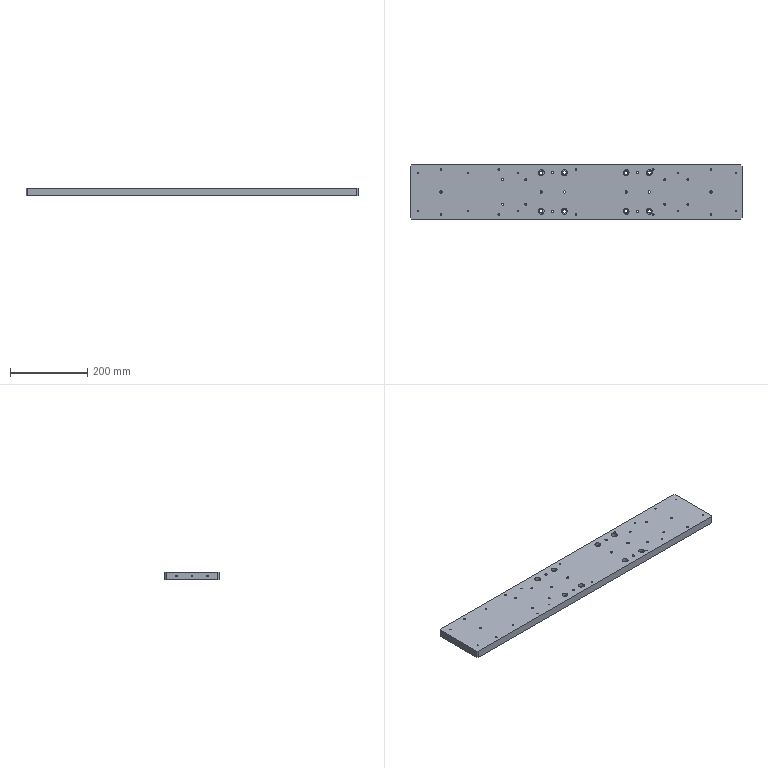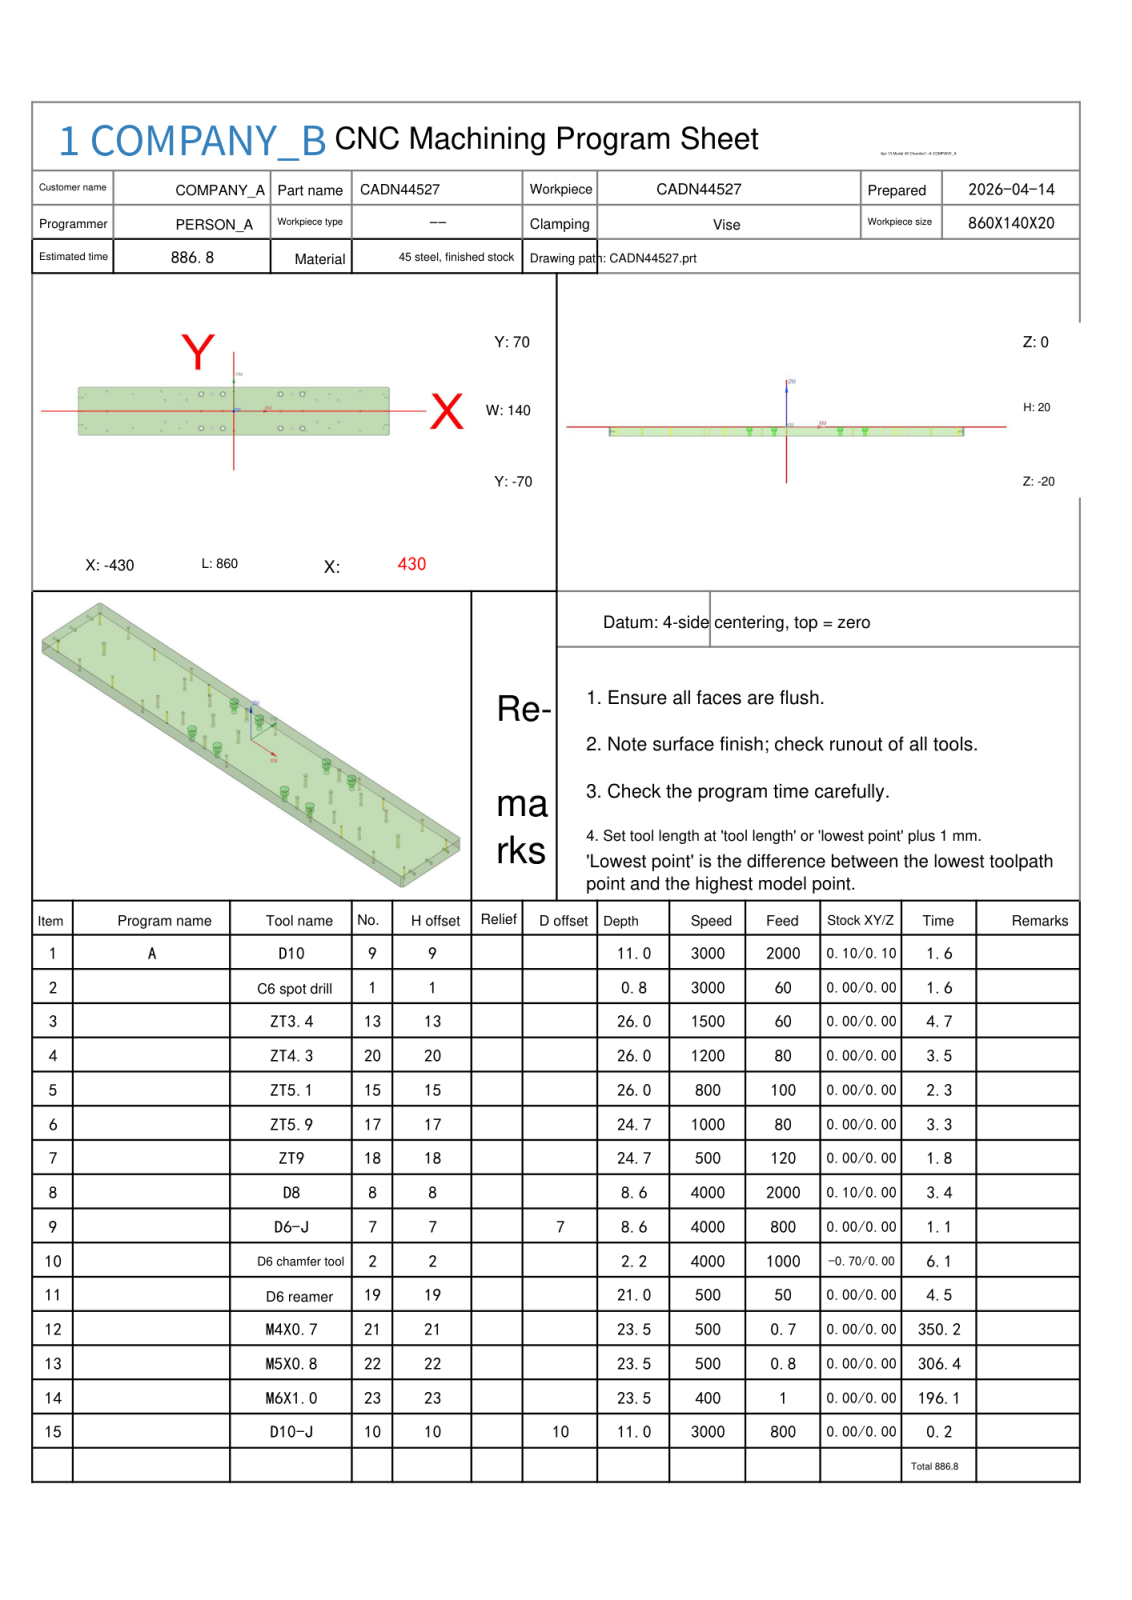NC program | NX | posted by the shop | part box 860 x 140 x 20 mm
Whole program, first 1720 of 2058 lines:
%
O0001
(Machine time: 1706.62 MIN)
(===Total Tool:15===)
(T9=D10     D=10.  R=0.   D-  H09 Z=-11.  )
(T1=C6 spot drill   D=6.   R=0.   D-  H01 Z=-0.8  )
(T13=ZT3.4  D=3.4  DR_a=118 D-  H13 Z=-26.  )
(T20=ZT4.3  D=4.3  DR_a=118 D-  H20 Z=-26.  )
(T15=ZT5.1  D=5.1  DR_a=118 D-  H15 Z=-26.  )
(T17=ZT5.9  D=5.9  DR_a=120 D-  H17 Z=-24.7 )
(T18=ZT9    D=9.   DR_a=118 D-  H18 Z=-24.7 )
(T8=D8      D=8.   R=0.   D-  H08 Z=-8.6  )
(T7=D6-J    D=6.   R=0.   D7  H07 Z=-8.6  )
(T2=D6 chamfer tool   D=6.   R=0.   D-  H02 Z=-2.2  )
(T19=D6 reamer   D=6.   DR_a=180 D-  H19 Z=-21.  )
(T21=M4X0.7 D=3.3  DR_a=180 D-  H21 Z=-23.5 )
(T22=M5X0.8 D=4.2  DR_a=180 D-  H22 Z=-23.5 )
(T23=M6X1.0 D=5.   DR_a=180 D-  H23 Z=-23.5 )
(T10=D10-J  D=10.  R=0.   D10 H10 Z=-11.  )
G80 G90 G17 G49 G40
G91 G28 Z0
M01
N1 T09 M06
(D10  D=10. R=0. H=09 ce=0.10 di=0.10)
G00 G90 G54 X-440.1 Y64.112 M03 S3000
G43 H09 Z50.
M08
Z-.344
G01 X-433.606 Y70.606 F2000.
X-430.606 Y73.606
X-424.112 Y80.1
G00 Z-.688
G01 X-430.606 Y73.606
X-433.606 Y70.606
X-440.1 Y64.112
G00 Z-1.031
G01 X-433.606 Y70.606
X-430.606 Y73.606
X-424.112 Y80.1
G00 Z-1.375
G01 X-430.606 Y73.606
X-433.606 Y70.606
X-440.1 Y64.112
G00 Z-1.719
G01 X-433.606 Y70.606
X-430.606 Y73.606
X-424.112 Y80.1
G00 Z-2.063
G01 X-430.606 Y73.606
X-433.606 Y70.606
X-440.1 Y64.112
G00 Z-2.406
G01 X-433.606 Y70.606
X-430.606 Y73.606
X-424.112 Y80.1
G00 Z-2.75
G01 X-430.606 Y73.606
X-433.606 Y70.606
X-440.1 Y64.112
G00 Z-3.094
G01 X-433.606 Y70.606
X-430.606 Y73.606
X-424.112 Y80.1
G00 Z-3.438
G01 X-430.606 Y73.606
X-433.606 Y70.606
X-440.1 Y64.112
G00 Z-3.781
G01 X-433.606 Y70.606
X-430.606 Y73.606
X-424.112 Y80.1
G00 Z-4.125
G01 X-430.606 Y73.606
X-433.606 Y70.606
X-440.1 Y64.112
G00 Z-4.469
G01 X-433.606 Y70.606
X-430.606 Y73.606
X-424.112 Y80.1
G00 Z-4.813
G01 X-430.606 Y73.606
X-433.606 Y70.606
X-440.1 Y64.112
G00 Z-5.156
G01 X-433.606 Y70.606
X-430.606 Y73.606
X-424.112 Y80.1
G00 Z-5.5
G01 X-430.606 Y73.606
X-433.606 Y70.606
X-440.1 Y64.112
G00 Z-5.844
G01 X-433.606 Y70.606
X-430.606 Y73.606
X-424.112 Y80.1
G00 Z-6.188
G01 X-430.606 Y73.606
X-433.606 Y70.606
X-440.1 Y64.112
G00 Z-6.531
G01 X-433.606 Y70.606
X-430.606 Y73.606
X-424.112 Y80.1
G00 Z-6.875
G01 X-430.606 Y73.606
X-433.606 Y70.606
X-440.1 Y64.112
G00 Z-7.219
G01 X-433.606 Y70.606
X-430.606 Y73.606
X-424.112 Y80.1
G00 Z-7.563
G01 X-430.606 Y73.606
X-433.606 Y70.606
X-440.1 Y64.112
G00 Z-7.906
G01 X-433.606 Y70.606
X-430.606 Y73.606
X-424.112 Y80.1
G00 Z-8.25
G01 X-430.606 Y73.606
X-433.606 Y70.606
X-440.1 Y64.112
G00 Z-8.594
G01 X-433.606 Y70.606
X-430.606 Y73.606
X-424.112 Y80.1
G00 Z-8.938
G01 X-430.606 Y73.606
X-433.606 Y70.606
X-440.1 Y64.112
G00 Z-9.281
G01 X-433.606 Y70.606
X-430.606 Y73.606
X-424.112 Y80.1
G00 Z-9.625
G01 X-430.606 Y73.606
X-433.606 Y70.606
X-440.1 Y64.112
G00 Z-9.969
G01 X-433.606 Y70.606
X-430.606 Y73.606
X-424.112 Y80.1
G00 Z-10.313
G01 X-430.606 Y73.606
X-433.606 Y70.606
X-440.1 Y64.112
G00 Z-10.656
G01 X-433.606 Y70.606
X-430.606 Y73.606
X-424.112 Y80.1
G00 Z-11.
G01 X-430.606 Y73.606
X-433.606 Y70.606
X-440.1 Y64.112
G00 Z50.
X-424.112 Y-80.1
Z-.344
G01 X-430.606 Y-73.606
X-433.606 Y-70.606
X-440.1 Y-64.112
G00 Z-.688
G01 X-433.606 Y-70.606
X-430.606 Y-73.606
X-424.112 Y-80.1
G00 Z-1.031
G01 X-430.606 Y-73.606
X-433.606 Y-70.606
X-440.1 Y-64.112
G00 Z-1.375
G01 X-433.606 Y-70.606
X-430.606 Y-73.606
X-424.112 Y-80.1
G00 Z-1.719
G01 X-430.606 Y-73.606
X-433.606 Y-70.606
X-440.1 Y-64.112
G00 Z-2.063
G01 X-433.606 Y-70.606
X-430.606 Y-73.606
X-424.112 Y-80.1
G00 Z-2.406
G01 X-430.606 Y-73.606
X-433.606 Y-70.606
X-440.1 Y-64.112
G00 Z-2.75
G01 X-433.606 Y-70.606
X-430.606 Y-73.606
X-424.112 Y-80.1
G00 Z-3.094
G01 X-430.606 Y-73.606
X-433.606 Y-70.606
X-440.1 Y-64.112
G00 Z-3.438
G01 X-433.606 Y-70.606
X-430.606 Y-73.606
X-424.112 Y-80.1
G00 Z-3.781
G01 X-430.606 Y-73.606
X-433.606 Y-70.606
X-440.1 Y-64.112
G00 Z-4.125
G01 X-433.606 Y-70.606
X-430.606 Y-73.606
X-424.112 Y-80.1
G00 Z-4.469
G01 X-430.606 Y-73.606
X-433.606 Y-70.606
X-440.1 Y-64.112
G00 Z-4.813
G01 X-433.606 Y-70.606
X-430.606 Y-73.606
X-424.112 Y-80.1
G00 Z-5.156
G01 X-430.606 Y-73.606
X-433.606 Y-70.606
X-440.1 Y-64.112
G00 Z-5.5
G01 X-433.606 Y-70.606
X-430.606 Y-73.606
X-424.112 Y-80.1
G00 Z-5.844
G01 X-430.606 Y-73.606
X-433.606 Y-70.606
X-440.1 Y-64.112
G00 Z-6.188
G01 X-433.606 Y-70.606
X-430.606 Y-73.606
X-424.112 Y-80.1
G00 Z-6.531
G01 X-430.606 Y-73.606
X-433.606 Y-70.606
X-440.1 Y-64.112
G00 Z-6.875
G01 X-433.606 Y-70.606
X-430.606 Y-73.606
X-424.112 Y-80.1
G00 Z-7.219
G01 X-430.606 Y-73.606
X-433.606 Y-70.606
X-440.1 Y-64.112
G00 Z-7.563
G01 X-433.606 Y-70.606
X-430.606 Y-73.606
X-424.112 Y-80.1
G00 Z-7.906
G01 X-430.606 Y-73.606
X-433.606 Y-70.606
X-440.1 Y-64.112
G00 Z-8.25
G01 X-433.606 Y-70.606
X-430.606 Y-73.606
X-424.112 Y-80.1
G00 Z-8.594
G01 X-430.606 Y-73.606
X-433.606 Y-70.606
X-440.1 Y-64.112
G00 Z-8.938
G01 X-433.606 Y-70.606
X-430.606 Y-73.606
X-424.112 Y-80.1
G00 Z-9.281
G01 X-430.606 Y-73.606
X-433.606 Y-70.606
X-440.1 Y-64.112
G00 Z-9.625
G01 X-433.606 Y-70.606
X-430.606 Y-73.606
X-424.112 Y-80.1
G00 Z-9.969
G01 X-430.606 Y-73.606
X-433.606 Y-70.606
X-440.1 Y-64.112
G00 Z-10.313
G01 X-433.606 Y-70.606
X-430.606 Y-73.606
X-424.112 Y-80.1
G00 Z-10.656
G01 X-430.606 Y-73.606
X-433.606 Y-70.606
X-440.1 Y-64.112
G00 Z-11.
G01 X-433.606 Y-70.606
X-430.606 Y-73.606
X-424.112 Y-80.1
G00 Z50.
X440.1 Y-64.112
Z-.344
G01 X433.606 Y-70.606
X430.606 Y-73.606
X424.112 Y-80.1
G00 Z-.688
G01 X430.606 Y-73.606
X433.606 Y-70.606
X440.1 Y-64.112
G00 Z-1.031
G01 X433.606 Y-70.606
X430.606 Y-73.606
X424.112 Y-80.1
G00 Z-1.375
G01 X430.606 Y-73.606
X433.606 Y-70.606
X440.1 Y-64.112
G00 Z-1.719
G01 X433.606 Y-70.606
X430.606 Y-73.606
X424.112 Y-80.1
G00 Z-2.063
G01 X430.606 Y-73.606
X433.606 Y-70.606
X440.1 Y-64.112
G00 Z-2.406
G01 X433.606 Y-70.606
X430.606 Y-73.606
X424.112 Y-80.1
G00 Z-2.75
G01 X430.606 Y-73.606
X433.606 Y-70.606
X440.1 Y-64.112
G00 Z-3.094
G01 X433.606 Y-70.606
X430.606 Y-73.606
X424.112 Y-80.1
G00 Z-3.438
G01 X430.606 Y-73.606
X433.606 Y-70.606
X440.1 Y-64.112
G00 Z-3.781
G01 X433.606 Y-70.606
X430.606 Y-73.606
X424.112 Y-80.1
G00 Z-4.125
G01 X430.606 Y-73.606
X433.606 Y-70.606
X440.1 Y-64.112
G00 Z-4.469
G01 X433.606 Y-70.606
X430.606 Y-73.606
X424.112 Y-80.1
G00 Z-4.813
G01 X430.606 Y-73.606
X433.606 Y-70.606
X440.1 Y-64.112
G00 Z-5.156
G01 X433.606 Y-70.606
X430.606 Y-73.606
X424.112 Y-80.1
G00 Z-5.5
G01 X430.606 Y-73.606
X433.606 Y-70.606
X440.1 Y-64.112
G00 Z-5.844
G01 X433.606 Y-70.606
X430.606 Y-73.606
X424.112 Y-80.1
G00 Z-6.188
G01 X430.606 Y-73.606
X433.606 Y-70.606
X440.1 Y-64.112
G00 Z-6.531
G01 X433.606 Y-70.606
X430.606 Y-73.606
X424.112 Y-80.1
G00 Z-6.875
G01 X430.606 Y-73.606
X433.606 Y-70.606
X440.1 Y-64.112
G00 Z-7.219
G01 X433.606 Y-70.606
X430.606 Y-73.606
X424.112 Y-80.1
G00 Z-7.563
G01 X430.606 Y-73.606
X433.606 Y-70.606
X440.1 Y-64.112
G00 Z-7.906
G01 X433.606 Y-70.606
X430.606 Y-73.606
X424.112 Y-80.1
G00 Z-8.25
G01 X430.606 Y-73.606
X433.606 Y-70.606
X440.1 Y-64.112
G00 Z-8.594
G01 X433.606 Y-70.606
X430.606 Y-73.606
X424.112 Y-80.1
G00 Z-8.938
G01 X430.606 Y-73.606
X433.606 Y-70.606
X440.1 Y-64.112
G00 Z-9.281
G01 X433.606 Y-70.606
X430.606 Y-73.606
X424.112 Y-80.1
G00 Z-9.625
G01 X430.606 Y-73.606
X433.606 Y-70.606
X440.1 Y-64.112
G00 Z-9.969
G01 X433.606 Y-70.606
X430.606 Y-73.606
X424.112 Y-80.1
G00 Z-10.313
G01 X430.606 Y-73.606
X433.606 Y-70.606
X440.1 Y-64.112
G00 Z-10.656
G01 X433.606 Y-70.606
X430.606 Y-73.606
X424.112 Y-80.1
G00 Z-11.
G01 X430.606 Y-73.606
X433.606 Y-70.606
X440.1 Y-64.112
G00 Z50.
X424.112 Y80.1
Z-.344
G01 X430.606 Y73.606
X433.606 Y70.606
X440.1 Y64.112
G00 Z-.688
G01 X433.606 Y70.606
X430.606 Y73.606
X424.112 Y80.1
G00 Z-1.031
G01 X430.606 Y73.606
X433.606 Y70.606
X440.1 Y64.112
G00 Z-1.375
G01 X433.606 Y70.606
X430.606 Y73.606
X424.112 Y80.1
G00 Z-1.719
G01 X430.606 Y73.606
X433.606 Y70.606
X440.1 Y64.112
G00 Z-2.063
G01 X433.606 Y70.606
X430.606 Y73.606
X424.112 Y80.1
G00 Z-2.406
G01 X430.606 Y73.606
X433.606 Y70.606
X440.1 Y64.112
G00 Z-2.75
G01 X433.606 Y70.606
X430.606 Y73.606
X424.112 Y80.1
G00 Z-3.094
G01 X430.606 Y73.606
X433.606 Y70.606
X440.1 Y64.112
G00 Z-3.438
G01 X433.606 Y70.606
X430.606 Y73.606
X424.112 Y80.1
G00 Z-3.781
G01 X430.606 Y73.606
X433.606 Y70.606
X440.1 Y64.112
G00 Z-4.125
G01 X433.606 Y70.606
X430.606 Y73.606
X424.112 Y80.1
G00 Z-4.469
G01 X430.606 Y73.606
X433.606 Y70.606
X440.1 Y64.112
G00 Z-4.813
G01 X433.606 Y70.606
X430.606 Y73.606
X424.112 Y80.1
G00 Z-5.156
G01 X430.606 Y73.606
X433.606 Y70.606
X440.1 Y64.112
G00 Z-5.5
G01 X433.606 Y70.606
X430.606 Y73.606
X424.112 Y80.1
G00 Z-5.844
G01 X430.606 Y73.606
X433.606 Y70.606
X440.1 Y64.112
G00 Z-6.188
G01 X433.606 Y70.606
X430.606 Y73.606
X424.112 Y80.1
G00 Z-6.531
G01 X430.606 Y73.606
X433.606 Y70.606
X440.1 Y64.112
G00 Z-6.875
G01 X433.606 Y70.606
X430.606 Y73.606
X424.112 Y80.1
G00 Z-7.219
G01 X430.606 Y73.606
X433.606 Y70.606
X440.1 Y64.112
G00 Z-7.563
G01 X433.606 Y70.606
X430.606 Y73.606
X424.112 Y80.1
G00 Z-7.906
G01 X430.606 Y73.606
X433.606 Y70.606
X440.1 Y64.112
G00 Z-8.25
G01 X433.606 Y70.606
X430.606 Y73.606
X424.112 Y80.1
G00 Z-8.594
G01 X430.606 Y73.606
X433.606 Y70.606
X440.1 Y64.112
G00 Z-8.938
G01 X433.606 Y70.606
X430.606 Y73.606
X424.112 Y80.1
G00 Z-9.281
G01 X430.606 Y73.606
X433.606 Y70.606
X440.1 Y64.112
G00 Z-9.625
G01 X433.606 Y70.606
X430.606 Y73.606
X424.112 Y80.1
G00 Z-9.969
G01 X430.606 Y73.606
X433.606 Y70.606
X440.1 Y64.112
G00 Z-10.313
G01 X433.606 Y70.606
X430.606 Y73.606
X424.112 Y80.1
G00 Z-10.656
G01 X430.606 Y73.606
X433.606 Y70.606
X440.1 Y64.112
G00 Z-11.
G01 X433.606 Y70.606
X430.606 Y73.606
X424.112 Y80.1
G00 Z50.
G91 G28 Z0.0
M05
M09
G91 G28 Z0.0
M01
N2 T01 M06
(C6 spot drill  D=6. R=0. H=01 ce=0.00 di=0.10)
G00 G90 G54 X190. Y0.0 M03 S3000
G43 H01 Z50.
M08
G98 G81 X190. Y0.0 Z-.8 R1. F60.
X130.
Y50.
X160.
X190.
X200. Y58.
X230. Y32.
X265. Y50.
X290. Y32.
X350. Y0.0
Y58.
X415. Y50.
Y-50.
X350. Y-58.
X290. Y-32.
X265. Y-50.
X230. Y-32.
X200. Y-58.
X190. Y-50.
X160.
X130.
X0.0 Y-58.
X-30. Y-50.
X-60.
X-90.
Y0.0
X-130. Y-32.
X-150. Y-50.
X-190. Y-32.
X-200. Y-58.
X-280. Y-50.
X-350. Y-58.
X-410. Y-50.
X-350. Y0.0
X-410. Y50.
X-350. Y58.
X-280. Y50.
X-200. Y58.
X-190. Y32.
X-150. Y50.
X-130. Y32.
X-90. Y50.
X-60.
X-30.
X0.0 Y58.
X-30. Y0.0
G80
G00 Z50.
G91 G28 Z0.0
M05
M09
G91 G28 Z0.0
M01
N3 T13 M06
(ZT3.4 D=3.4 DR_a=118 H=13)
G00 G90 G54 X415. Y-50. M03 S1500
G43 H13 Z50.
M08
G98 G83 X415. Y-50. Z-26. R1. F60. Q1.
Y50.
X265.
Y-50.
X-150.
Y50.
X-280.
Y-50.
X-410.
Y50.
G80
G00 Z50.
G91 G28 Z0.0
M05
M09
G91 G28 Z0.0
M01
N4 T20 M06
(ZT4.3 D=4.3 DR_a=118 H=20)
G00 G90 G54 X350. Y58. M03 S1200
G43 H20 Z50.
M08
G98 G83 X350. Y58. Z-26. R1. F80. Q1.5
Y-58.
X200.
Y58.
X0.0
Y-58.
X-200.
Y58.
X-350.
Y-58.
G80
G00 Z50.
G91 G28 Z0.0
M05
M09
G91 G28 Z0.0
M01
N5 T15 M06
(ZT5.1 D=5.1 DR_a=118 H=15)
G00 G90 G54 X-130. Y-32. M03 S800
G43 H15 Z50.
M08
G98 G83 X-130. Y-32. Z-26. R1. F100. Q2.
X-190.
Y32.
X-130.
X230.
X290.
Y-32.
X230.
G80
G00 Z50.
G91 G28 Z0.0
M05
M09
G91 G28 Z0.0
M01
N6 T17 M06
(ZT5.9 D=5.9 DR_a=120 H=17)
G00 G90 G54 X-350. Y0.0 M03 S1000
G43 H17 Z50.
M08
G98 G83 X-350. Y0.0 Z-24.703 R1. F80. Q1.
X-90.
X-60. Y50.
X-30. Y0.0
X-60. Y-50.
X160.
X130. Y0.0
X160. Y50.
X190. Y0.0
X350.
G80
G00 Z50.
G91 G28 Z0.0
M05
M09
G91 G28 Z0.0
M01
N7 T18 M06
(ZT9 D=9. DR_a=118 H=18)
G00 G90 G54 X-30. Y-50. M03 S500
G43 H18 Z50.
M08
G98 G83 X-30. Y-50. Z-24.704 R1. F120. Q2.
X-90.
Y50.
X-30.
X130.
X190.
Y-50.
X130.
G80
G00 Z50.
G91 G28 Z0.0
M05
M09
G91 G28 Z0.0
M01
N8 T08 M06
(D8  D=8. R=0. H=08 ce=0.10 di=0.00)
G00 G90 G54 X-30. Y-50. M03 S4000
G43 H08 Z50.
M08
Z.5
G03 X-28.3 Y-51.7 I1.7 J0.0 F2000.
X-26.6 Y-50. I0.0 J1.7
X-26.6 Y-50. Z.25 I-3.4 J0.0
X-26.6 Y-50. Z0.0 I-3.4 J0.0
X-26.6 Y-50. Z-.25 I-3.4 J0.0
X-26.6 Y-50. Z-.5 I-3.4 J0.0
X-26.6 Y-50. Z-.75 I-3.4 J0.0
X-26.6 Y-50. Z-1. I-3.4 J0.0
X-26.6 Y-50. Z-1.25 I-3.4 J0.0
X-26.6 Y-50. Z-1.5 I-3.4 J0.0
X-26.6 Y-50. Z-1.75 I-3.4 J0.0
X-26.6 Y-50. Z-2. I-3.4 J0.0
X-26.6 Y-50. Z-2.25 I-3.4 J0.0
X-26.6 Y-50. Z-2.5 I-3.4 J0.0
X-26.6 Y-50. Z-2.75 I-3.4 J0.0
X-26.6 Y-50. Z-3. I-3.4 J0.0
X-26.6 Y-50. Z-3.25 I-3.4 J0.0
X-26.6 Y-50. Z-3.5 I-3.4 J0.0
X-26.6 Y-50. Z-3.75 I-3.4 J0.0
X-26.6 Y-50. Z-4. I-3.4 J0.0
X-26.6 Y-50. Z-4.25 I-3.4 J0.0
X-26.6 Y-50. Z-4.5 I-3.4 J0.0
X-26.6 Y-50. Z-4.75 I-3.4 J0.0
X-26.6 Y-50. Z-5. I-3.4 J0.0
X-26.6 Y-50. Z-5.25 I-3.4 J0.0
X-26.6 Y-50. Z-5.5 I-3.4 J0.0
X-26.6 Y-50. Z-5.75 I-3.4 J0.0
X-26.6 Y-50. Z-6. I-3.4 J0.0
X-26.6 Y-50. Z-6.25 I-3.4 J0.0
X-26.6 Y-50. Z-6.5 I-3.4 J0.0
X-26.6 Y-50. Z-6.75 I-3.4 J0.0
X-26.6 Y-50. Z-7. I-3.4 J0.0
X-26.6 Y-50. Z-7.25 I-3.4 J0.0
X-26.6 Y-50. Z-7.5 I-3.4 J0.0
X-26.6 Y-50. Z-7.75 I-3.4 J0.0
X-26.6 Y-50. Z-8. I-3.4 J0.0
X-26.6 Y-50. Z-8.25 I-3.4 J0.0
X-26.6 Y-50. Z-8.5 I-3.4 J0.0
X-32.751 Y-48.002 Z-8.6 I-3.4 J0.0
X-33.4 Y-50. I2.751 J-1.998
X-30. Y-53.4 I3.4 J0.0
X-26.6 Y-50. I0.0 J3.4
X-30. Y-46.6 I-3.4 J0.0
X-32.751 Y-48.002 I0.0 J-3.4
X-33.075 Y-49.001 I1.375 J-.999
X-31.375 Y-50.701 I1.7 J0.0
X-30. Y-50. I0.0 J1.7
G00 Z50.
X-90.
Z.5
G03 X-88.3 Y-51.7 I1.7 J0.0
X-86.6 Y-50. I0.0 J1.7
X-86.6 Y-50. Z.25 I-3.4 J0.0
X-86.6 Y-50. Z0.0 I-3.4 J0.0
X-86.6 Y-50. Z-.25 I-3.4 J0.0
X-86.6 Y-50. Z-.5 I-3.4 J0.0
X-86.6 Y-50. Z-.75 I-3.4 J0.0
X-86.6 Y-50. Z-1. I-3.4 J0.0
X-86.6 Y-50. Z-1.25 I-3.4 J0.0
X-86.6 Y-50. Z-1.5 I-3.4 J0.0
X-86.6 Y-50. Z-1.75 I-3.4 J0.0
X-86.6 Y-50. Z-2. I-3.4 J0.0
X-86.6 Y-50. Z-2.25 I-3.4 J0.0
X-86.6 Y-50. Z-2.5 I-3.4 J0.0
X-86.6 Y-50. Z-2.75 I-3.4 J0.0
X-86.6 Y-50. Z-3. I-3.4 J0.0
X-86.6 Y-50. Z-3.25 I-3.4 J0.0
X-86.6 Y-50. Z-3.5 I-3.4 J0.0
X-86.6 Y-50. Z-3.75 I-3.4 J0.0
X-86.6 Y-50. Z-4. I-3.4 J0.0
X-86.6 Y-50. Z-4.25 I-3.4 J0.0
X-86.6 Y-50. Z-4.5 I-3.4 J0.0
X-86.6 Y-50. Z-4.75 I-3.4 J0.0
X-86.6 Y-50. Z-5. I-3.4 J0.0
X-86.6 Y-50. Z-5.25 I-3.4 J0.0
X-86.6 Y-50. Z-5.5 I-3.4 J0.0
X-86.6 Y-50. Z-5.75 I-3.4 J0.0
X-86.6 Y-50. Z-6. I-3.4 J0.0
X-86.6 Y-50. Z-6.25 I-3.4 J0.0
X-86.6 Y-50. Z-6.5 I-3.4 J0.0
X-86.6 Y-50. Z-6.75 I-3.4 J0.0
X-86.6 Y-50. Z-7. I-3.4 J0.0
X-86.6 Y-50. Z-7.25 I-3.4 J0.0
X-86.6 Y-50. Z-7.5 I-3.4 J0.0
X-86.6 Y-50. Z-7.75 I-3.4 J0.0
X-86.6 Y-50. Z-8. I-3.4 J0.0
X-86.6 Y-50. Z-8.25 I-3.4 J0.0
X-86.6 Y-50. Z-8.5 I-3.4 J0.0
X-92.751 Y-48.002 Z-8.6 I-3.4 J0.0
X-93.4 Y-50. I2.751 J-1.998
X-90. Y-53.4 I3.4 J0.0
X-86.6 Y-50. I0.0 J3.4
X-90. Y-46.6 I-3.4 J0.0
X-92.751 Y-48.002 I0.0 J-3.4
X-93.075 Y-49.001 I1.375 J-.999
X-91.375 Y-50.701 I1.7 J0.0
X-90. Y-50. I0.0 J1.7
G00 Z50.
Y50.
Z.5
G03 X-88.3 Y48.3 I1.7 J0.0
X-86.6 Y50. I0.0 J1.7
X-86.6 Y50. Z.25 I-3.4 J0.0
X-86.6 Y50. Z0.0 I-3.4 J0.0
X-86.6 Y50. Z-.25 I-3.4 J0.0
X-86.6 Y50. Z-.5 I-3.4 J0.0
X-86.6 Y50. Z-.75 I-3.4 J0.0
X-86.6 Y50. Z-1. I-3.4 J0.0
X-86.6 Y50. Z-1.25 I-3.4 J0.0
X-86.6 Y50. Z-1.5 I-3.4 J0.0
X-86.6 Y50. Z-1.75 I-3.4 J0.0
X-86.6 Y50. Z-2. I-3.4 J0.0
X-86.6 Y50. Z-2.25 I-3.4 J0.0
X-86.6 Y50. Z-2.5 I-3.4 J0.0
X-86.6 Y50. Z-2.75 I-3.4 J0.0
X-86.6 Y50. Z-3. I-3.4 J0.0
X-86.6 Y50. Z-3.25 I-3.4 J0.0
X-86.6 Y50. Z-3.5 I-3.4 J0.0
X-86.6 Y50. Z-3.75 I-3.4 J0.0
X-86.6 Y50. Z-4. I-3.4 J0.0
X-86.6 Y50. Z-4.25 I-3.4 J0.0
X-86.6 Y50. Z-4.5 I-3.4 J0.0
X-86.6 Y50. Z-4.75 I-3.4 J0.0
X-86.6 Y50. Z-5. I-3.4 J0.0
X-86.6 Y50. Z-5.25 I-3.4 J0.0
X-86.6 Y50. Z-5.5 I-3.4 J0.0
X-86.6 Y50. Z-5.75 I-3.4 J0.0
X-86.6 Y50. Z-6. I-3.4 J0.0
X-86.6 Y50. Z-6.25 I-3.4 J0.0
X-86.6 Y50. Z-6.5 I-3.4 J0.0
X-86.6 Y50. Z-6.75 I-3.4 J0.0
X-86.6 Y50. Z-7. I-3.4 J0.0
X-86.6 Y50. Z-7.25 I-3.4 J0.0
X-86.6 Y50. Z-7.5 I-3.4 J0.0
X-86.6 Y50. Z-7.75 I-3.4 J0.0
X-86.6 Y50. Z-8. I-3.4 J0.0
X-86.6 Y50. Z-8.25 I-3.4 J0.0
X-86.6 Y50. Z-8.5 I-3.4 J0.0
X-92.751 Y51.998 Z-8.6 I-3.4 J0.0
X-93.4 Y50. I2.751 J-1.998
X-90. Y46.6 I3.4 J0.0
X-86.6 Y50. I0.0 J3.4
X-90. Y53.4 I-3.4 J0.0
X-92.751 Y51.998 I0.0 J-3.4
X-93.075 Y50.999 I1.375 J-.999
X-91.375 Y49.299 I1.7 J0.0
X-90. Y50. I0.0 J1.7
G00 Z50.
X-30.
Z.5
G03 X-28.3 Y48.3 I1.7 J0.0
X-26.6 Y50. I0.0 J1.7
X-26.6 Y50. Z.25 I-3.4 J0.0
X-26.6 Y50. Z0.0 I-3.4 J0.0
X-26.6 Y50. Z-.25 I-3.4 J0.0
X-26.6 Y50. Z-.5 I-3.4 J0.0
X-26.6 Y50. Z-.75 I-3.4 J0.0
X-26.6 Y50. Z-1. I-3.4 J0.0
X-26.6 Y50. Z-1.25 I-3.4 J0.0
X-26.6 Y50. Z-1.5 I-3.4 J0.0
X-26.6 Y50. Z-1.75 I-3.4 J0.0
X-26.6 Y50. Z-2. I-3.4 J0.0
X-26.6 Y50. Z-2.25 I-3.4 J0.0
X-26.6 Y50. Z-2.5 I-3.4 J0.0
X-26.6 Y50. Z-2.75 I-3.4 J0.0
X-26.6 Y50. Z-3. I-3.4 J0.0
X-26.6 Y50. Z-3.25 I-3.4 J0.0
X-26.6 Y50. Z-3.5 I-3.4 J0.0
X-26.6 Y50. Z-3.75 I-3.4 J0.0
X-26.6 Y50. Z-4. I-3.4 J0.0
X-26.6 Y50. Z-4.25 I-3.4 J0.0
X-26.6 Y50. Z-4.5 I-3.4 J0.0
X-26.6 Y50. Z-4.75 I-3.4 J0.0
X-26.6 Y50. Z-5. I-3.4 J0.0
X-26.6 Y50. Z-5.25 I-3.4 J0.0
X-26.6 Y50. Z-5.5 I-3.4 J0.0
X-26.6 Y50. Z-5.75 I-3.4 J0.0
X-26.6 Y50. Z-6. I-3.4 J0.0
X-26.6 Y50. Z-6.25 I-3.4 J0.0
X-26.6 Y50. Z-6.5 I-3.4 J0.0
X-26.6 Y50. Z-6.75 I-3.4 J0.0
X-26.6 Y50. Z-7. I-3.4 J0.0
X-26.6 Y50. Z-7.25 I-3.4 J0.0
X-26.6 Y50. Z-7.5 I-3.4 J0.0
X-26.6 Y50. Z-7.75 I-3.4 J0.0
X-26.6 Y50. Z-8. I-3.4 J0.0
X-26.6 Y50. Z-8.25 I-3.4 J0.0
X-26.6 Y50. Z-8.5 I-3.4 J0.0
X-32.751 Y51.998 Z-8.6 I-3.4 J0.0
X-33.4 Y50. I2.751 J-1.998
X-30. Y46.6 I3.4 J0.0
X-26.6 Y50. I0.0 J3.4
X-30. Y53.4 I-3.4 J0.0
X-32.751 Y51.998 I0.0 J-3.4
X-33.075 Y50.999 I1.375 J-.999
X-31.375 Y49.299 I1.7 J0.0
X-30. Y50. I0.0 J1.7
G00 Z50.
X130.
Z.5
G03 X131.7 Y48.3 I1.7 J0.0
X133.4 Y50. I0.0 J1.7
X133.4 Y50. Z.25 I-3.4 J0.0
X133.4 Y50. Z0.0 I-3.4 J0.0
X133.4 Y50. Z-.25 I-3.4 J0.0
X133.4 Y50. Z-.5 I-3.4 J0.0
X133.4 Y50. Z-.75 I-3.4 J0.0
X133.4 Y50. Z-1. I-3.4 J0.0
X133.4 Y50. Z-1.25 I-3.4 J0.0
X133.4 Y50. Z-1.5 I-3.4 J0.0
X133.4 Y50. Z-1.75 I-3.4 J0.0
X133.4 Y50. Z-2. I-3.4 J0.0
X133.4 Y50. Z-2.25 I-3.4 J0.0
X133.4 Y50. Z-2.5 I-3.4 J0.0
X133.4 Y50. Z-2.75 I-3.4 J0.0
X133.4 Y50. Z-3. I-3.4 J0.0
X133.4 Y50. Z-3.25 I-3.4 J0.0
X133.4 Y50. Z-3.5 I-3.4 J0.0
X133.4 Y50. Z-3.75 I-3.4 J0.0
X133.4 Y50. Z-4. I-3.4 J0.0
X133.4 Y50. Z-4.25 I-3.4 J0.0
X133.4 Y50. Z-4.5 I-3.4 J0.0
X133.4 Y50. Z-4.75 I-3.4 J0.0
X133.4 Y50. Z-5. I-3.4 J0.0
X133.4 Y50. Z-5.25 I-3.4 J0.0
X133.4 Y50. Z-5.5 I-3.4 J0.0
X133.4 Y50. Z-5.75 I-3.4 J0.0
X133.4 Y50. Z-6. I-3.4 J0.0
X133.4 Y50. Z-6.25 I-3.4 J0.0
X133.4 Y50. Z-6.5 I-3.4 J0.0
X133.4 Y50. Z-6.75 I-3.4 J0.0
X133.4 Y50. Z-7. I-3.4 J0.0
X133.4 Y50. Z-7.25 I-3.4 J0.0
X133.4 Y50. Z-7.5 I-3.4 J0.0
X133.4 Y50. Z-7.75 I-3.4 J0.0
X133.4 Y50. Z-8. I-3.4 J0.0
X133.4 Y50. Z-8.25 I-3.4 J0.0
X133.4 Y50. Z-8.5 I-3.4 J0.0
X127.249 Y51.998 Z-8.6 I-3.4 J0.0
X126.6 Y50. I2.751 J-1.998
X130. Y46.6 I3.4 J0.0
X133.4 Y50. I0.0 J3.4
X130. Y53.4 I-3.4 J0.0
X127.249 Y51.998 I0.0 J-3.4
X126.925 Y50.999 I1.375 J-.999
X128.625 Y49.299 I1.7 J0.0
X130. Y50. I0.0 J1.7
G00 Z50.
X190.
Z.5
G03 X191.7 Y48.3 I1.7 J0.0
X193.4 Y50. I0.0 J1.7
X193.4 Y50. Z.25 I-3.4 J0.0
X193.4 Y50. Z0.0 I-3.4 J0.0
X193.4 Y50. Z-.25 I-3.4 J0.0
X193.4 Y50. Z-.5 I-3.4 J0.0
X193.4 Y50. Z-.75 I-3.4 J0.0
X193.4 Y50. Z-1. I-3.4 J0.0
X193.4 Y50. Z-1.25 I-3.4 J0.0
X193.4 Y50. Z-1.5 I-3.4 J0.0
X193.4 Y50. Z-1.75 I-3.4 J0.0
X193.4 Y50. Z-2. I-3.4 J0.0
X193.4 Y50. Z-2.25 I-3.4 J0.0
X193.4 Y50. Z-2.5 I-3.4 J0.0
X193.4 Y50. Z-2.75 I-3.4 J0.0
X193.4 Y50. Z-3. I-3.4 J0.0
X193.4 Y50. Z-3.25 I-3.4 J0.0
X193.4 Y50. Z-3.5 I-3.4 J0.0
X193.4 Y50. Z-3.75 I-3.4 J0.0
X193.4 Y50. Z-4. I-3.4 J0.0
X193.4 Y50. Z-4.25 I-3.4 J0.0
X193.4 Y50. Z-4.5 I-3.4 J0.0
X193.4 Y50. Z-4.75 I-3.4 J0.0
X193.4 Y50. Z-5. I-3.4 J0.0
X193.4 Y50. Z-5.25 I-3.4 J0.0
X193.4 Y50. Z-5.5 I-3.4 J0.0
X193.4 Y50. Z-5.75 I-3.4 J0.0
X193.4 Y50. Z-6. I-3.4 J0.0
X193.4 Y50. Z-6.25 I-3.4 J0.0
X193.4 Y50. Z-6.5 I-3.4 J0.0
X193.4 Y50. Z-6.75 I-3.4 J0.0
X193.4 Y50. Z-7. I-3.4 J0.0
X193.4 Y50. Z-7.25 I-3.4 J0.0
X193.4 Y50. Z-7.5 I-3.4 J0.0
X193.4 Y50. Z-7.75 I-3.4 J0.0
X193.4 Y50. Z-8. I-3.4 J0.0
X193.4 Y50. Z-8.25 I-3.4 J0.0
X193.4 Y50. Z-8.5 I-3.4 J0.0
X187.249 Y51.998 Z-8.6 I-3.4 J0.0
X186.6 Y50. I2.751 J-1.998
X190. Y46.6 I3.4 J0.0
X193.4 Y50. I0.0 J3.4
X190. Y53.4 I-3.4 J0.0
X187.249 Y51.998 I0.0 J-3.4
X186.925 Y50.999 I1.375 J-.999
X188.625 Y49.299 I1.7 J0.0
X190. Y50. I0.0 J1.7
G00 Z50.
Y-50.
Z.5
G03 X191.7 Y-51.7 I1.7 J0.0
X193.4 Y-50. I0.0 J1.7
X193.4 Y-50. Z.25 I-3.4 J0.0
X193.4 Y-50. Z0.0 I-3.4 J0.0
X193.4 Y-50. Z-.25 I-3.4 J0.0
X193.4 Y-50. Z-.5 I-3.4 J0.0
X193.4 Y-50. Z-.75 I-3.4 J0.0
X193.4 Y-50. Z-1. I-3.4 J0.0
X193.4 Y-50. Z-1.25 I-3.4 J0.0
X193.4 Y-50. Z-1.5 I-3.4 J0.0
X193.4 Y-50. Z-1.75 I-3.4 J0.0
X193.4 Y-50. Z-2. I-3.4 J0.0
X193.4 Y-50. Z-2.25 I-3.4 J0.0
X193.4 Y-50. Z-2.5 I-3.4 J0.0
X193.4 Y-50. Z-2.75 I-3.4 J0.0
X193.4 Y-50. Z-3. I-3.4 J0.0
X193.4 Y-50. Z-3.25 I-3.4 J0.0
X193.4 Y-50. Z-3.5 I-3.4 J0.0
X193.4 Y-50. Z-3.75 I-3.4 J0.0
X193.4 Y-50. Z-4. I-3.4 J0.0
X193.4 Y-50. Z-4.25 I-3.4 J0.0
X193.4 Y-50. Z-4.5 I-3.4 J0.0
X193.4 Y-50. Z-4.75 I-3.4 J0.0
X193.4 Y-50. Z-5. I-3.4 J0.0
X193.4 Y-50. Z-5.25 I-3.4 J0.0
X193.4 Y-50. Z-5.5 I-3.4 J0.0
X193.4 Y-50. Z-5.75 I-3.4 J0.0
X193.4 Y-50. Z-6. I-3.4 J0.0
X193.4 Y-50. Z-6.25 I-3.4 J0.0
X193.4 Y-50. Z-6.5 I-3.4 J0.0
X193.4 Y-50. Z-6.75 I-3.4 J0.0
X193.4 Y-50. Z-7. I-3.4 J0.0
X193.4 Y-50. Z-7.25 I-3.4 J0.0
X193.4 Y-50. Z-7.5 I-3.4 J0.0
X193.4 Y-50. Z-7.75 I-3.4 J0.0
X193.4 Y-50. Z-8. I-3.4 J0.0
X193.4 Y-50. Z-8.25 I-3.4 J0.0
X193.4 Y-50. Z-8.5 I-3.4 J0.0
X187.249 Y-48.002 Z-8.6 I-3.4 J0.0
X186.6 Y-50. I2.751 J-1.998
X190. Y-53.4 I3.4 J0.0
X193.4 Y-50. I0.0 J3.4
X190. Y-46.6 I-3.4 J0.0
X187.249 Y-48.002 I0.0 J-3.4
X186.925 Y-49.001 I1.375 J-.999
X188.625 Y-50.701 I1.7 J0.0
X190. Y-50. I0.0 J1.7
G00 Z50.
X130.
Z.5
G03 X131.7 Y-51.7 I1.7 J0.0
X133.4 Y-50. I0.0 J1.7
X133.4 Y-50. Z.25 I-3.4 J0.0
X133.4 Y-50. Z0.0 I-3.4 J0.0
X133.4 Y-50. Z-.25 I-3.4 J0.0
X133.4 Y-50. Z-.5 I-3.4 J0.0
X133.4 Y-50. Z-.75 I-3.4 J0.0
X133.4 Y-50. Z-1. I-3.4 J0.0
X133.4 Y-50. Z-1.25 I-3.4 J0.0
X133.4 Y-50. Z-1.5 I-3.4 J0.0
X133.4 Y-50. Z-1.75 I-3.4 J0.0
X133.4 Y-50. Z-2. I-3.4 J0.0
X133.4 Y-50. Z-2.25 I-3.4 J0.0
X133.4 Y-50. Z-2.5 I-3.4 J0.0
X133.4 Y-50. Z-2.75 I-3.4 J0.0
X133.4 Y-50. Z-3. I-3.4 J0.0
X133.4 Y-50. Z-3.25 I-3.4 J0.0
X133.4 Y-50. Z-3.5 I-3.4 J0.0
X133.4 Y-50. Z-3.75 I-3.4 J0.0
X133.4 Y-50. Z-4. I-3.4 J0.0
X133.4 Y-50. Z-4.25 I-3.4 J0.0
X133.4 Y-50. Z-4.5 I-3.4 J0.0
X133.4 Y-50. Z-4.75 I-3.4 J0.0
X133.4 Y-50. Z-5. I-3.4 J0.0
X133.4 Y-50. Z-5.25 I-3.4 J0.0
X133.4 Y-50. Z-5.5 I-3.4 J0.0
X133.4 Y-50. Z-5.75 I-3.4 J0.0
X133.4 Y-50. Z-6. I-3.4 J0.0
X133.4 Y-50. Z-6.25 I-3.4 J0.0
X133.4 Y-50. Z-6.5 I-3.4 J0.0
X133.4 Y-50. Z-6.75 I-3.4 J0.0
X133.4 Y-50. Z-7. I-3.4 J0.0
X133.4 Y-50. Z-7.25 I-3.4 J0.0
X133.4 Y-50. Z-7.5 I-3.4 J0.0
X133.4 Y-50. Z-7.75 I-3.4 J0.0
X133.4 Y-50. Z-8. I-3.4 J0.0
X133.4 Y-50. Z-8.25 I-3.4 J0.0
X133.4 Y-50. Z-8.5 I-3.4 J0.0
X127.249 Y-48.002 Z-8.6 I-3.4 J0.0
X126.6 Y-50. I2.751 J-1.998
X130. Y-53.4 I3.4 J0.0
X133.4 Y-50. I0.0 J3.4
X130. Y-46.6 I-3.4 J0.0
X127.249 Y-48.002 I0.0 J-3.4
X126.925 Y-49.001 I1.375 J-.999
X128.625 Y-50.701 I1.7 J0.0
X130. Y-50. I0.0 J1.7
G00 Z50.
G91 G28 Z0.0
M05
M09
G91 G28 Z0.0
M01
N9 T07 M06
(D6-J  D=6. R=0. H=07 ce=0.00 di=0.00)
G00 G90 G54 X-30. Y-50. M03 S4000
G43 H07 Z50.
M08
Z.5
G41 D07
G01 X-29.206 Y-51.153 F800.
G03 X-27.532 Y-52.032 I1.674 J1.153
X-25.5 Y-50. I0.0 J2.032
X-25.5 Y-50. Z-4.5 I-4.5 J0.0
X-28.084 Y-54.072 Z-8.6 I-4.5 J0.0
X-25.5 Y-50. I-1.916 J4.072
X-30. Y-45.5 I-4.5 J0.0
X-34.5 Y-50. I0.0 J-4.5
X-30. Y-54.5 I4.5 J0.0
X-28.084 Y-54.072 I0.0 J4.5
X-26.917 Y-52.233 I-.865 J1.839
X-28.619 Y-50.228 I-2.032 J0.0
G01 G40 X-30. Y-50.
G00 Z50.
X-90.
Z.5
G41 D07
G01 X-89.206 Y-51.153
G03 X-87.532 Y-52.032 I1.674 J1.153
X-85.5 Y-50. I0.0 J2.032
X-85.5 Y-50. Z-4.5 I-4.5 J0.0
X-88.084 Y-54.072 Z-8.6 I-4.5 J0.0
X-85.5 Y-50. I-1.916 J4.072
X-90. Y-45.5 I-4.5 J0.0
X-94.5 Y-50. I0.0 J-4.5
X-90. Y-54.5 I4.5 J0.0
X-88.084 Y-54.072 I0.0 J4.5
X-86.917 Y-52.233 I-.865 J1.839
X-88.619 Y-50.228 I-2.032 J0.0
G01 G40 X-90. Y-50.
G00 Z50.
Y50.
Z.5
G41 D07
G01 X-89.206 Y48.847
G03 X-87.532 Y47.968 I1.674 J1.153
X-85.5 Y50. I0.0 J2.032
X-85.5 Y50. Z-4.5 I-4.5 J0.0
X-88.084 Y45.928 Z-8.6 I-4.5 J0.0
X-85.5 Y50. I-1.916 J4.072
X-90. Y54.5 I-4.5 J0.0
X-94.5 Y50. I0.0 J-4.5
X-90. Y45.5 I4.5 J0.0
X-88.084 Y45.928 I0.0 J4.5
X-86.917 Y47.767 I-.865 J1.839
X-88.619 Y49.772 I-2.032 J0.0
G01 G40 X-90. Y50.
G00 Z50.
X-30.
Z.5
G41 D07
G01 X-29.206 Y48.847
G03 X-27.532 Y47.968 I1.674 J1.153
X-25.5 Y50. I0.0 J2.032
X-25.5 Y50. Z-4.5 I-4.5 J0.0
X-28.084 Y45.928 Z-8.6 I-4.5 J0.0
X-25.5 Y50. I-1.916 J4.072
X-30. Y54.5 I-4.5 J0.0
X-34.5 Y50. I0.0 J-4.5
X-30. Y45.5 I4.5 J0.0
X-28.084 Y45.928 I0.0 J4.5
X-26.917 Y47.767 I-.865 J1.839
X-28.619 Y49.772 I-2.032 J0.0
G01 G40 X-30. Y50.
G00 Z50.
X130.
Z.5
G41 D07
G01 X130.794 Y48.847
G03 X132.468 Y47.968 I1.674 J1.153
X134.5 Y50. I0.0 J2.032
X134.5 Y50. Z-4.5 I-4.5 J0.0
X131.916 Y45.928 Z-8.6 I-4.5 J0.0
X134.5 Y50. I-1.916 J4.072
X130. Y54.5 I-4.5 J0.0
X125.5 Y50. I0.0 J-4.5
X130. Y45.5 I4.5 J0.0
X131.916 Y45.928 I0.0 J4.5
X133.083 Y47.767 I-.865 J1.839
X131.381 Y49.772 I-2.032 J0.0
G01 G40 X130. Y50.
G00 Z50.
X190.
Z.5
G41 D07
G01 X190.794 Y48.847
G03 X192.468 Y47.968 I1.674 J1.153
X194.5 Y50. I0.0 J2.032
X194.5 Y50. Z-4.5 I-4.5 J0.0
X191.916 Y45.928 Z-8.6 I-4.5 J0.0
X194.5 Y50. I-1.916 J4.072
X190. Y54.5 I-4.5 J0.0
X185.5 Y50. I0.0 J-4.5
X190. Y45.5 I4.5 J0.0
X191.916 Y45.928 I0.0 J4.5
X193.083 Y47.767 I-.865 J1.839
X191.381 Y49.772 I-2.032 J0.0
G01 G40 X190. Y50.
G00 Z50.
Y-50.
Z.5
G41 D07
G01 X190.794 Y-51.153
G03 X192.468 Y-52.032 I1.674 J1.153
X194.5 Y-50. I0.0 J2.032
X194.5 Y-50. Z-4.5 I-4.5 J0.0
X191.916 Y-54.072 Z-8.6 I-4.5 J0.0
X194.5 Y-50. I-1.916 J4.072
X190. Y-45.5 I-4.5 J0.0
X185.5 Y-50. I0.0 J-4.5
X190. Y-54.5 I4.5 J0.0
X191.916 Y-54.072 I0.0 J4.5
X193.083 Y-52.233 I-.865 J1.839
X191.381 Y-50.228 I-2.032 J0.0
G01 G40 X190. Y-50.
G00 Z50.
X130.
Z.5
G41 D07
G01 X130.794 Y-51.153
G03 X132.468 Y-52.032 I1.674 J1.153
X134.5 Y-50. I0.0 J2.032
X134.5 Y-50. Z-4.5 I-4.5 J0.0
X131.916 Y-54.072 Z-8.6 I-4.5 J0.0
X134.5 Y-50. I-1.916 J4.072
X130. Y-45.5 I-4.5 J0.0
X125.5 Y-50. I0.0 J-4.5
X130. Y-54.5 I4.5 J0.0
X131.916 Y-54.072 I0.0 J4.5
X133.083 Y-52.233 I-.865 J1.839
X131.381 Y-50.228 I-2.032 J0.0
G01 G40 X130. Y-50.
G00 Z50.
G91 G28 Z0.0
M05
M09
G91 G28 Z0.0
M01
N10 T02 M06
(D6 chamfer tool  D=6. R=0. H=02 ce=0.00 di=0.00)
G00 G90 G54 X415. Y-50. M03 S4000
G43 H02 Z50.
M08
G98 G81 X415. Y-50. Z-2.2 R3. F80.
Y50.
X265.
Y-50.
X-150.
Y50.
X-280.
Y-50.
X-410.
Y50.
G80
G00 Z50.
G00 G90 X350.093 Y57.306 M03 S4000
Z50.
Z-.5
G01 Z-1. F200.
X350.2 Y56.5
G03 X351.7 Y58. I0.0 J1.5
X350. Y59.7 I-1.7 J0.0
X348.3 Y58. I0.0 J-1.7
X350. Y56.3 I1.7 J0.0
X351.7 Y58. I0.0 J1.7
X350.2 Y59.5 I-1.5 J0.0
G01 X350.093 Y58.694
Z-.5
G00 Z50.
Y-58.694
Z-.5
G01 Z-1.
X350.2 Y-59.5
G03 X351.7 Y-58. I0.0 J1.5
X350. Y-56.3 I-1.7 J0.0
X348.3 Y-58. I0.0 J-1.7
X350. Y-59.7 I1.7 J0.0
X351.7 Y-58. I0.0 J1.7
X350.2 Y-56.5 I-1.5 J0.0
G01 X350.093 Y-57.306
Z-.5
G00 Z50.
X200.093 Y-58.694
Z-.5
G01 Z-1.
X200.2 Y-59.5
G03 X201.7 Y-58. I0.0 J1.5
X200. Y-56.3 I-1.7 J0.0
X198.3 Y-58. I0.0 J-1.7
X200. Y-59.7 I1.7 J0.0
X201.7 Y-58. I0.0 J1.7
X200.2 Y-56.5 I-1.5 J0.0
G01 X200.093 Y-57.306
Z-.5
G00 Z50.
Y57.306
Z-.5
G01 Z-1.
X200.2 Y56.5
G03 X201.7 Y58. I0.0 J1.5
X200. Y59.7 I-1.7 J0.0
X198.3 Y58. I0.0 J-1.7
X200. Y56.3 I1.7 J0.0
X201.7 Y58. I0.0 J1.7
X200.2 Y59.5 I-1.5 J0.0
G01 X200.093 Y58.694
Z-.5
G00 Z50.
X.093 Y57.306
Z-.5
G01 Z-1.
X.2 Y56.5
G03 X1.7 Y58. I0.0 J1.5
X0.0 Y59.7 I-1.7 J0.0
X-1.7 Y58. I0.0 J-1.7
X0.0 Y56.3 I1.7 J0.0
X1.7 Y58. I0.0 J1.7
X.2 Y59.5 I-1.5 J0.0
G01 X.093 Y58.694
Z-.5
G00 Z50.
Y-58.694
Z-.5
G01 Z-1.
X.2 Y-59.5
G03 X1.7 Y-58. I0.0 J1.5
X0.0 Y-56.3 I-1.7 J0.0
X-1.7 Y-58. I0.0 J-1.7
X0.0 Y-59.7 I1.7 J0.0
X1.7 Y-58. I0.0 J1.7
X.2 Y-56.5 I-1.5 J0.0
G01 X.093 Y-57.306
Z-.5
G00 Z50.
X-199.907 Y-58.694
Z-.5
G01 Z-1.
X-199.8 Y-59.5
G03 X-198.3 Y-58. I0.0 J1.5
X-200. Y-56.3 I-1.7 J0.0
X-201.7 Y-58. I0.0 J-1.7
X-200. Y-59.7 I1.7 J0.0
X-198.3 Y-58. I0.0 J1.7
X-199.8 Y-56.5 I-1.5 J0.0
G01 X-199.907 Y-57.306
Z-.5
G00 Z50.
Y57.306
Z-.5
G01 Z-1.
X-199.8 Y56.5
G03 X-198.3 Y58. I0.0 J1.5
X-200. Y59.7 I-1.7 J0.0
X-201.7 Y58. I0.0 J-1.7
X-200. Y56.3 I1.7 J0.0
X-198.3 Y58. I0.0 J1.7
X-199.8 Y59.5 I-1.5 J0.0
G01 X-199.907 Y58.694
Z-.5
G00 Z50.
X-349.907 Y57.306
Z-.5
G01 Z-1.
X-349.8 Y56.5
G03 X-348.3 Y58. I0.0 J1.5
X-350. Y59.7 I-1.7 J0.0
X-351.7 Y58. I0.0 J-1.7
X-350. Y56.3 I1.7 J0.0
X-348.3 Y58. I0.0 J1.7
X-349.8 Y59.5 I-1.5 J0.0
G01 X-349.907 Y58.694
Z-.5
G00 Z50.
Y-58.694
Z-.5
G01 Z-1.
X-349.8 Y-59.5
G03 X-348.3 Y-58. I0.0 J1.5
X-350. Y-56.3 I-1.7 J0.0
X-351.7 Y-58. I0.0 J-1.7
X-350. Y-59.7 I1.7 J0.0
X-348.3 Y-58. I0.0 J1.7
X-349.8 Y-56.5 I-1.5 J0.0
G01 X-349.907 Y-57.306
Z-.5
G00 Z50.
G00 G90 X230.409 Y30.979 M03 S4000
Z50.
Z-.6
G01 Z-1.1 F300.
X230.6 Y30.5
G03 X232.1 Y32. I0.0 J1.5
X230. Y34.1 I-2.1 J0.0
X227.9 Y32. I0.0 J-2.1
X230. Y29.9 I2.1 J0.0
X232.1 Y32. I0.0 J2.1
X230.6 Y33.5 I-1.5 J0.0
G01 X230.409 Y33.021
Z-.6
G00 Z50.
X290.409 Y30.979
Z-.6
G01 Z-1.1
X290.6 Y30.5
G03 X292.1 Y32. I0.0 J1.5
X290. Y34.1 I-2.1 J0.0
X287.9 Y32. I0.0 J-2.1
X290. Y29.9 I2.1 J0.0
X292.1 Y32. I0.0 J2.1
X290.6 Y33.5 I-1.5 J0.0
G01 X290.409 Y33.021
Z-.6
G00 Z50.
Y-33.021
Z-.6
G01 Z-1.1
X290.6 Y-33.5
G03 X292.1 Y-32. I0.0 J1.5
X290. Y-29.9 I-2.1 J0.0
X287.9 Y-32. I0.0 J-2.1
X290. Y-34.1 I2.1 J0.0
X292.1 Y-32. I0.0 J2.1
X290.6 Y-30.5 I-1.5 J0.0
G01 X290.409 Y-30.979
Z-.6
G00 Z50.
X230.409 Y-33.021
Z-.6
G01 Z-1.1
X230.6 Y-33.5
G03 X232.1 Y-32. I0.0 J1.5
X230. Y-29.9 I-2.1 J0.0
X227.9 Y-32. I0.0 J-2.1
X230. Y-34.1 I2.1 J0.0
X232.1 Y-32. I0.0 J2.1
X230.6 Y-30.5 I-1.5 J0.0
G01 X230.409 Y-30.979
Z-.6
G00 Z50.
X-129.591 Y-33.021
Z-.6
G01 Z-1.1
X-129.4 Y-33.5
G03 X-127.9 Y-32. I0.0 J1.5
X-130. Y-29.9 I-2.1 J0.0
X-132.1 Y-32. I0.0 J-2.1
X-130. Y-34.1 I2.1 J0.0
X-127.9 Y-32. I0.0 J2.1
X-129.4 Y-30.5 I-1.5 J0.0
G01 X-129.591 Y-30.979
Z-.6
G00 Z50.
X-189.591 Y-33.021
Z-.6
G01 Z-1.1
X-189.4 Y-33.5
G03 X-187.9 Y-32. I0.0 J1.5
X-190. Y-29.9 I-2.1 J0.0
X-192.1 Y-32. I0.0 J-2.1
X-190. Y-34.1 I2.1 J0.0
X-187.9 Y-32. I0.0 J2.1
X-189.4 Y-30.5 I-1.5 J0.0
G01 X-189.591 Y-30.979
Z-.6
G00 Z50.
Y30.979
Z-.6
G01 Z-1.1
X-189.4 Y30.5
G03 X-187.9 Y32. I0.0 J1.5
X-190. Y34.1 I-2.1 J0.0
X-192.1 Y32. I0.0 J-2.1
X-190. Y29.9 I2.1 J0.0
X-187.9 Y32. I0.0 J2.1
X-189.4 Y33.5 I-1.5 J0.0
G01 X-189.591 Y33.021
Z-.6
G00 Z50.
X-129.591 Y30.979
Z-.6
G01 Z-1.1
X-129.4 Y30.5
G03 X-127.9 Y32. I0.0 J1.5
X-130. Y34.1 I-2.1 J0.0
X-132.1 Y32. I0.0 J-2.1
X-130. Y29.9 I2.1 J0.0
X-127.9 Y32. I0.0 J2.1
X-129.4 Y33.5 I-1.5 J0.0
G01 X-129.591 Y33.021
Z-.6
G00 Z50.
G00 G90 X-349.388 Y-1.147 M03 S4000
Z50.
Z-.5
G01 Z-1. F400.
X-349.2 Y-1.5
G03 X-347.7 Y0.0 I0.0 J1.5
X-350. Y2.3 I-2.3 J0.0
X-352.3 Y0.0 I0.0 J-2.3
X-350. Y-2.3 I2.3 J0.0
X-347.7 Y0.0 I0.0 J2.3
X-349.2 Y1.5 I-1.5 J0.0
G01 X-349.388 Y1.147
Z-.5
G00 Z50.
X-90.612
Z-.5
G01 Z-1.
X-90.8 Y1.5
G03 X-92.3 Y0.0 I0.0 J-1.5
X-90. Y-2.3 I2.3 J0.0
X-87.7 Y0.0 I0.0 J2.3
X-90. Y2.3 I-2.3 J0.0
X-92.3 Y0.0 I0.0 J-2.3
X-90.8 Y-1.5 I1.5 J0.0
G01 X-90.612 Y-1.147
Z-.5
G00 Z50.
X-60.612 Y51.147
Z-.5
G01 Z-1.
X-60.8 Y51.5
G03 X-62.3 Y50. I0.0 J-1.5
X-60. Y47.7 I2.3 J0.0
X-57.7 Y50. I0.0 J2.3
X-60. Y52.3 I-2.3 J0.0
X-62.3 Y50. I0.0 J-2.3
X-60.8 Y48.5 I1.5 J0.0
G01 X-60.612 Y48.853
Z-.5
G00 Z50.
Y-48.853
Z-.5
G01 Z-1.
X-60.8 Y-48.5
G03 X-62.3 Y-50. I0.0 J-1.5
X-60. Y-52.3 I2.3 J0.0
X-57.7 Y-50. I0.0 J2.3
X-60. Y-47.7 I-2.3 J0.0
X-62.3 Y-50. I0.0 J-2.3
X-60.8 Y-51.5 I1.5 J0.0
G01 X-60.612 Y-51.147
Z-.5
G00 Z50.
X-30.612 Y1.147
Z-.5
G01 Z-1.
X-30.8 Y1.5
G03 X-32.3 Y0.0 I0.0 J-1.5
X-30. Y-2.3 I2.3 J0.0
X-27.7 Y0.0 I0.0 J2.3
X-30. Y2.3 I-2.3 J0.0
X-32.3 Y0.0 I0.0 J-2.3
X-30.8 Y-1.5 I1.5 J0.0
G01 X-30.612 Y-1.147
Z-.5
G00 Z50.
X129.388 Y1.147
Z-.5
G01 Z-1.
X129.2 Y1.5
G03 X127.7 Y0.0 I0.0 J-1.5
X130. Y-2.3 I2.3 J0.0
X132.3 Y0.0 I0.0 J2.3
X130. Y2.3 I-2.3 J0.0
X127.7 Y0.0 I0.0 J-2.3
X129.2 Y-1.5 I1.5 J0.0
G01 X129.388 Y-1.147
Z-.5
G00 Z50.
X159.388 Y-48.853
Z-.5
G01 Z-1.
X159.2 Y-48.5
G03 X157.7 Y-50. I0.0 J-1.5
X160. Y-52.3 I2.3 J0.0
X162.3 Y-50. I0.0 J2.3
X160. Y-47.7 I-2.3 J0.0
X157.7 Y-50. I0.0 J-2.3
X159.2 Y-51.5 I1.5 J0.0
G01 X159.388 Y-51.147
Z-.5
G00 Z50.
Y51.147
Z-.5
G01 Z-1.
X159.2 Y51.5
G03 X157.7 Y50. I0.0 J-1.5
X160. Y47.7 I2.3 J0.0
X162.3 Y50. I0.0 J2.3
X160. Y52.3 I-2.3 J0.0
X157.7 Y50. I0.0 J-2.3
X159.2 Y48.5 I1.5 J0.0
G01 X159.388 Y48.853
Z-.5
G00 Z50.
X189.388 Y1.147
Z-.5
G01 Z-1.
X189.2 Y1.5
G03 X187.7 Y0.0 I0.0 J-1.5
X190. Y-2.3 I2.3 J0.0
X192.3 Y0.0 I0.0 J2.3
X190. Y2.3 I-2.3 J0.0
X187.7 Y0.0 I0.0 J-2.3
X189.2 Y-1.5 I1.5 J0.0
G01 X189.388 Y-1.147
Z-.5
G00 Z50.
X350.612
Z-.5
G01 Z-1.
X350.8 Y-1.5
G03 X352.3 Y0.0 I0.0 J1.5
X350. Y2.3 I-2.3 J0.0
X347.7 Y0.0 I0.0 J-2.3
X350. Y-2.3 I2.3 J0.0
X352.3 Y0.0 I0.0 J2.3
X350.8 Y1.5 I-1.5 J0.0
G01 X350.612 Y1.147
Z-.5
G00 Z50.
G00 G90 X-28.937 Y-56.719 M03 S4000
Z50.
Z2.5
G01 X-28.392 Y-56.61 Z2.297 F800.
X-27.859 Y-56.457 Z2.096
X-27.341 Y-56.262 Z1.894
X-26.841 Y-56.025 Z1.693
X-26.362 Y-55.748 Z1.492
X-25.906 Y-55.433 Z1.29
X-25.478 Y-55.083 Z1.089
X-25.08 Y-54.698 Z.887
X-24.714 Y-54.282 Z.686
X-24.383 Y-53.838 Z.484
X-24.09 Y-53.369 Z.283
X-23.835 Y-52.877 Z.081
X-23.622 Y-52.367 Z-.12
X-23.451 Y-51.84 Z-.322
X-23.323 Y-51.301 Z-.523
X-23.239 Y-50.754 Z-.725
X-23.2 Y-50.202 Z-.926
Y-50. Z-1.
G03 X-30. Y-43.2 I-6.8 J0.0
X-36.8 Y-50. I0.0 J-6.8
X-30. Y-56.8 I6.8 J0.0
X-23.2 Y-50. I0.0 J6.8
X-23.218 Y-49.5 I-6.8 J0.0
G01 Z1.5
G00 Z50.
X-88.937 Y-56.719
Z2.5
G01 X-88.392 Y-56.61 Z2.297
X-87.859 Y-56.457 Z2.096
X-87.341 Y-56.262 Z1.894
X-86.841 Y-56.025 Z1.693
X-86.362 Y-55.748 Z1.492
X-85.906 Y-55.433 Z1.29
X-85.478 Y-55.083 Z1.089
X-85.08 Y-54.698 Z.887
X-84.714 Y-54.282 Z.686
X-84.383 Y-53.838 Z.484
X-84.09 Y-53.369 Z.283
X-83.835 Y-52.877 Z.081
X-83.622 Y-52.367 Z-.12
X-83.451 Y-51.84 Z-.322
X-83.323 Y-51.301 Z-.523
X-83.239 Y-50.754 Z-.725
X-83.2 Y-50.202 Z-.926
Y-50. Z-1.
G03 X-90. Y-43.2 I-6.8 J0.0
X-96.8 Y-50. I0.0 J-6.8
X-90. Y-56.8 I6.8 J0.0
X-83.2 Y-50. I0.0 J6.8
X-83.218 Y-49.5 I-6.8 J0.0
G01 Z1.5
G00 Z50.
X-88.937 Y43.281
Z2.5
G01 X-88.392 Y43.39 Z2.297
X-87.859 Y43.543 Z2.096
X-87.341 Y43.738 Z1.894
X-86.841 Y43.975 Z1.693
X-86.362 Y44.252 Z1.492
X-85.906 Y44.567 Z1.29
X-85.478 Y44.917 Z1.089
X-85.08 Y45.302 Z.887
X-84.714 Y45.718 Z.686
X-84.383 Y46.162 Z.484